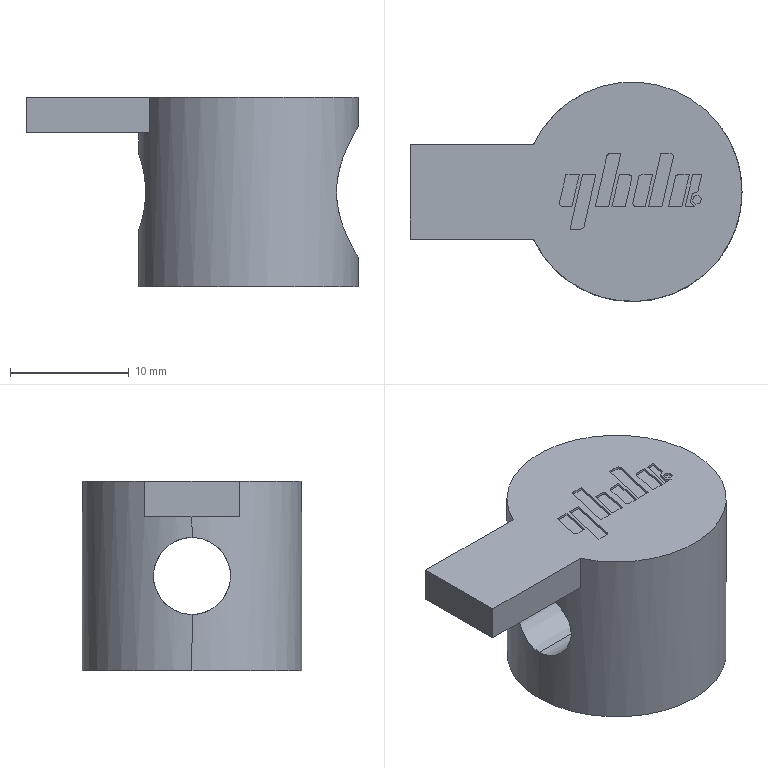Part | SolidWorks | features BaseBody 1 | 1 solid | 73 faces | box 28 x 18.5 x 16 mm | volume 3220 mm3 | plane 57 | cylinder 16 | commonest cylinder face diameters 0.562 x10 6.5 x2 11 x2 18.5 x2